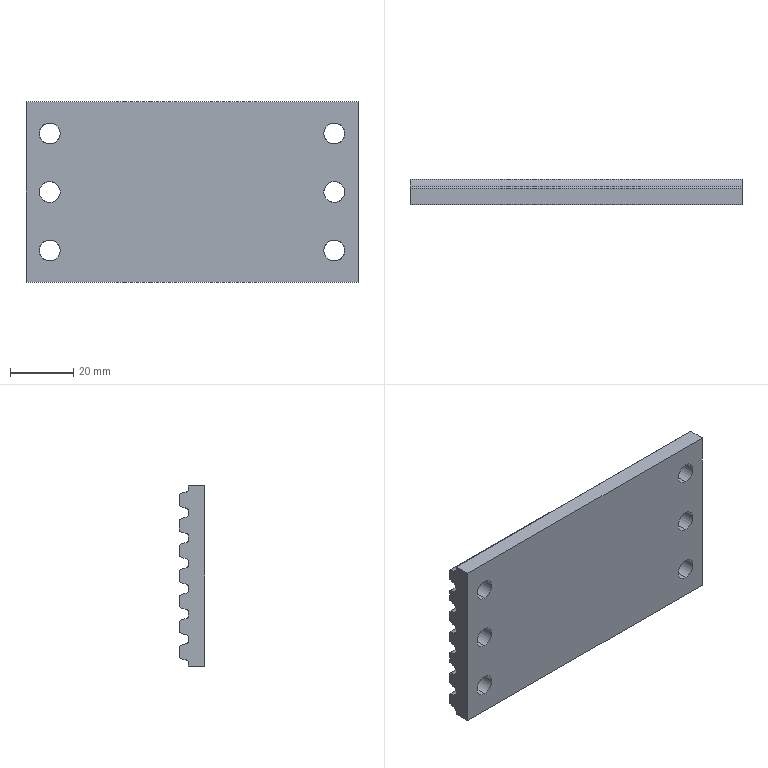Part | SolidWorks | features HoleWzd 1, WeldMemberFeat 1, WeldmentFeature 1 | 1 solid | 82 faces | box 105 x 8 x 57 mm | volume 39266 mm3 | cylinder 56 | plane 26 | commonest cylinder face diameters 1.6 x22 10.4 x22 6.6 x12